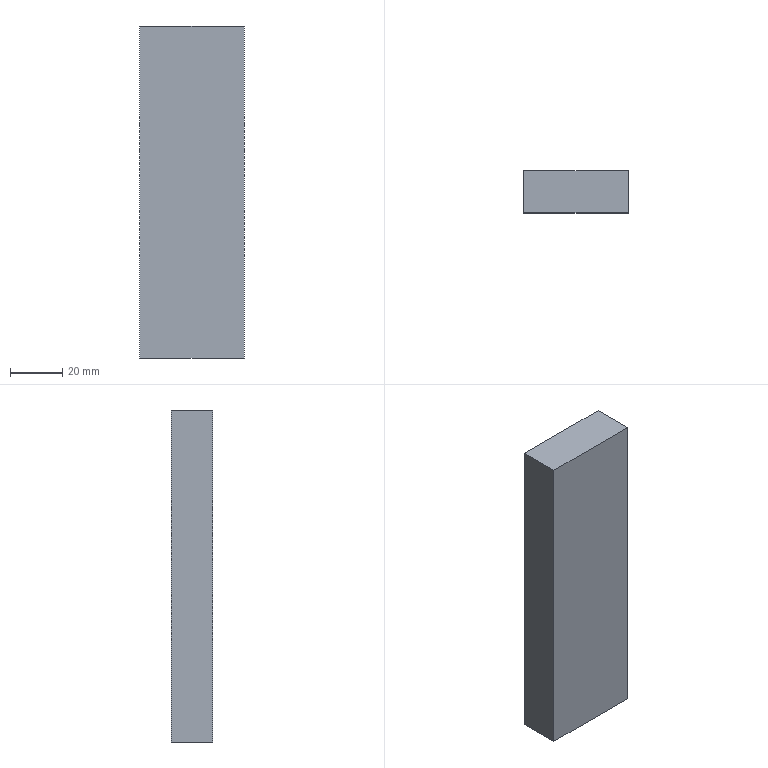Part | NX | features 5003_209_Plate 2 | 1 solid | 6 faces | box 40 x 16 x 127 mm | volume 81280 mm3 | plane 6
STEP:
#1=CARTESIAN_POINT('',(-148.775,-186.606,-154.));
#2=VERTEX_POINT('',#1);
#3=CARTESIAN_POINT('',(-148.775,-186.606,-27.));
#4=VERTEX_POINT('',#3);
#5=CARTESIAN_POINT('',(-148.775,-186.606,-105.5));
#6=DIRECTION('',(0.,0.,1.));
#7=VECTOR('',#6,1000.);
#8=LINE('',#5,#7);
#9=EDGE_CURVE('',#2,#4,#8,.T.);
#10=ORIENTED_EDGE('',*,*,#9,.T.);
#11=CARTESIAN_POINT('',(-188.775,-186.606,-27.));
#12=VERTEX_POINT('',#11);
#13=CARTESIAN_POINT('',(-196.775,-186.606,-27.));
#14=DIRECTION('',(1.,0.,0.));
#15=VECTOR('',#14,1000.);
#16=LINE('',#13,#15);
#17=EDGE_CURVE('',#4,#12,#16,.F.);
#18=ORIENTED_EDGE('',*,*,#17,.T.);
#19=CARTESIAN_POINT('',(-188.775,-186.606,-154.));
#20=VERTEX_POINT('',#19);
#21=CARTESIAN_POINT('',(-188.775,-186.606,-115.5));
#22=DIRECTION('',(0.,0.,-1.));
#23=VECTOR('',#22,1000.);
#24=LINE('',#21,#23);
#25=EDGE_CURVE('',#12,#20,#24,.T.);
#26=ORIENTED_EDGE('',*,*,#25,.T.);
#27=CARTESIAN_POINT('',(174.525,-186.606,-154.));
#28=DIRECTION('',(1.,0.,0.));
#29=VECTOR('',#28,1000.);
#30=LINE('',#27,#29);
#31=EDGE_CURVE('',#20,#2,#30,.T.);
#32=ORIENTED_EDGE('',*,*,#31,.T.);
#33=EDGE_LOOP('',(#10,#18,#26,#32));
#34=FACE_BOUND('',#33,.T.);
#35=CARTESIAN_POINT('',(-171.775,-186.606,-95.5));
#36=DIRECTION('',(0.,-1.,0.));
#37=DIRECTION('',(1.,0.,0.));
#38=AXIS2_PLACEMENT_3D('',#35,#36,#37);
#39=PLANE('',#38);
#40=ADVANCED_FACE('',(#34),#39,.T.);
#41=CARTESIAN_POINT('',(-148.775,-170.606,-27.));
#42=VERTEX_POINT('',#41);
#43=CARTESIAN_POINT('',(-188.775,-170.606,-27.));
#44=VERTEX_POINT('',#43);
#45=CARTESIAN_POINT('',(-196.775,-170.606,-27.));
#46=DIRECTION('',(-1.,0.,0.));
#47=VECTOR('',#46,1000.);
#48=LINE('',#45,#47);
#49=EDGE_CURVE('',#42,#44,#48,.T.);
#50=ORIENTED_EDGE('',*,*,#49,.F.);
#51=CARTESIAN_POINT('',(-148.775,-170.606,-154.));
#52=VERTEX_POINT('',#51);
#53=CARTESIAN_POINT('',(-148.775,-170.606,-105.5));
#54=DIRECTION('',(0.,0.,1.));
#55=VECTOR('',#54,1000.);
#56=LINE('',#53,#55);
#57=EDGE_CURVE('',#52,#42,#56,.T.);
#58=ORIENTED_EDGE('',*,*,#57,.F.);
#59=CARTESIAN_POINT('',(-188.775,-170.606,-154.));
#60=VERTEX_POINT('',#59);
#61=CARTESIAN_POINT('',(174.525,-170.606,-154.));
#62=DIRECTION('',(1.,0.,0.));
#63=VECTOR('',#62,1000.);
#64=LINE('',#61,#63);
#65=EDGE_CURVE('',#60,#52,#64,.T.);
#66=ORIENTED_EDGE('',*,*,#65,.F.);
#67=CARTESIAN_POINT('',(-188.775,-170.606,-115.5));
#68=DIRECTION('',(0.,0.,-1.));
#69=VECTOR('',#68,1000.);
#70=LINE('',#67,#69);
#71=EDGE_CURVE('',#44,#60,#70,.T.);
#72=ORIENTED_EDGE('',*,*,#71,.F.);
#73=EDGE_LOOP('',(#50,#58,#66,#72));
#74=FACE_BOUND('',#73,.T.);
#75=CARTESIAN_POINT('',(-171.775,-170.606,-95.5));
#76=DIRECTION('',(0.,-1.,0.));
#77=DIRECTION('',(1.,0.,0.));
#78=AXIS2_PLACEMENT_3D('',#75,#76,#77);
#79=PLANE('',#78);
#80=ADVANCED_FACE('',(#74),#79,.F.);
#81=ORIENTED_EDGE('',*,*,#17,.F.);
#82=CARTESIAN_POINT('',(-148.775,-186.606,-27.));
#83=DIRECTION('',(0.,-1.,0.));
#84=VECTOR('',#83,1000.);
#85=LINE('',#82,#84);
#86=EDGE_CURVE('',#42,#4,#85,.T.);
#87=ORIENTED_EDGE('',*,*,#86,.F.);
#88=ORIENTED_EDGE('',*,*,#49,.T.);
#89=CARTESIAN_POINT('',(-188.775,-474.612,-27.));
#90=DIRECTION('',(0.,1.,0.));
#91=VECTOR('',#90,1000.);
#92=LINE('',#89,#91);
#93=EDGE_CURVE('',#44,#12,#92,.F.);
#94=ORIENTED_EDGE('',*,*,#93,.T.);
#95=EDGE_LOOP('',(#81,#87,#88,#94));
#96=FACE_BOUND('',#95,.T.);
#97=CARTESIAN_POINT('',(-196.775,-474.612,-27.));
#98=DIRECTION('',(0.,0.,-1.));
#99=DIRECTION('',(0.,1.,0.));
#100=AXIS2_PLACEMENT_3D('',#97,#98,#99);
#101=PLANE('',#100);
#102=ADVANCED_FACE('',(#96),#101,.F.);
#103=ORIENTED_EDGE('',*,*,#25,.F.);
#104=ORIENTED_EDGE('',*,*,#93,.F.);
#105=ORIENTED_EDGE('',*,*,#71,.T.);
#106=CARTESIAN_POINT('',(-188.775,-11.,-154.));
#107=DIRECTION('',(0.,1.,0.));
#108=VECTOR('',#107,1000.);
#109=LINE('',#106,#108);
#110=EDGE_CURVE('',#20,#60,#109,.T.);
#111=ORIENTED_EDGE('',*,*,#110,.F.);
#112=EDGE_LOOP('',(#103,#104,#105,#111));
#113=FACE_BOUND('',#112,.T.);
#114=CARTESIAN_POINT('',(-188.775,-186.606,-115.5));
#115=DIRECTION('',(1.,0.,0.));
#116=DIRECTION('',(0.,1.,0.));
#117=AXIS2_PLACEMENT_3D('',#114,#115,#116);
#118=PLANE('',#117);
#119=ADVANCED_FACE('',(#113),#118,.F.);
#120=ORIENTED_EDGE('',*,*,#65,.T.);
#121=CARTESIAN_POINT('',(-148.775,-186.606,-154.));
#122=DIRECTION('',(0.,1.,0.));
#123=VECTOR('',#122,1000.);
#124=LINE('',#121,#123);
#125=EDGE_CURVE('',#2,#52,#124,.T.);
#126=ORIENTED_EDGE('',*,*,#125,.F.);
#127=ORIENTED_EDGE('',*,*,#31,.F.);
#128=ORIENTED_EDGE('',*,*,#110,.T.);
#129=EDGE_LOOP('',(#120,#126,#127,#128));
#130=FACE_BOUND('',#129,.T.);
#131=CARTESIAN_POINT('',(174.525,-11.,-154.));
#132=DIRECTION('',(0.,0.,1.));
#133=DIRECTION('',(-1.,0.,0.));
#134=AXIS2_PLACEMENT_3D('',#131,#132,#133);
#135=PLANE('',#134);
#136=ADVANCED_FACE('',(#130),#135,.F.);
#137=ORIENTED_EDGE('',*,*,#57,.T.);
#138=ORIENTED_EDGE('',*,*,#86,.T.);
#139=ORIENTED_EDGE('',*,*,#9,.F.);
#140=ORIENTED_EDGE('',*,*,#125,.T.);
#141=EDGE_LOOP('',(#137,#138,#139,#140));
#142=FACE_BOUND('',#141,.T.);
#143=CARTESIAN_POINT('',(-148.775,-186.606,-105.5));
#144=DIRECTION('',(-1.,0.,0.));
#145=DIRECTION('',(0.,0.,-1.));
#146=AXIS2_PLACEMENT_3D('',#143,#144,#145);
#147=PLANE('',#146);
#148=ADVANCED_FACE('',(#142),#147,.F.);
#149=CLOSED_SHELL('',(#40,#80,#102,#119,#136,#148));
#150=MANIFOLD_SOLID_BREP('',#149);
#151=(LENGTH_UNIT()NAMED_UNIT(*)SI_UNIT(.MILLI.,.METRE.));
#152=UNCERTAINTY_MEASURE_WITH_UNIT(LENGTH_MEASURE(0.00001),#151,'','');
#153=(NAMED_UNIT(*)PLANE_ANGLE_UNIT()SI_UNIT($,.RADIAN.));
#154=(NAMED_UNIT(*)SI_UNIT($,.STERADIAN.)SOLID_ANGLE_UNIT());
#155=(GEOMETRIC_REPRESENTATION_CONTEXT(3)GLOBAL_UNCERTAINTY_ASSIGNED_CONTEXT((#152))GLOBAL_UNIT_ASSIGNED_CONTEXT((#151,#153,#154))REPRESENTATION_CONTEXT('',''));
#156=ADVANCED_BREP_SHAPE_REPRESENTATION('',(#150),#155);